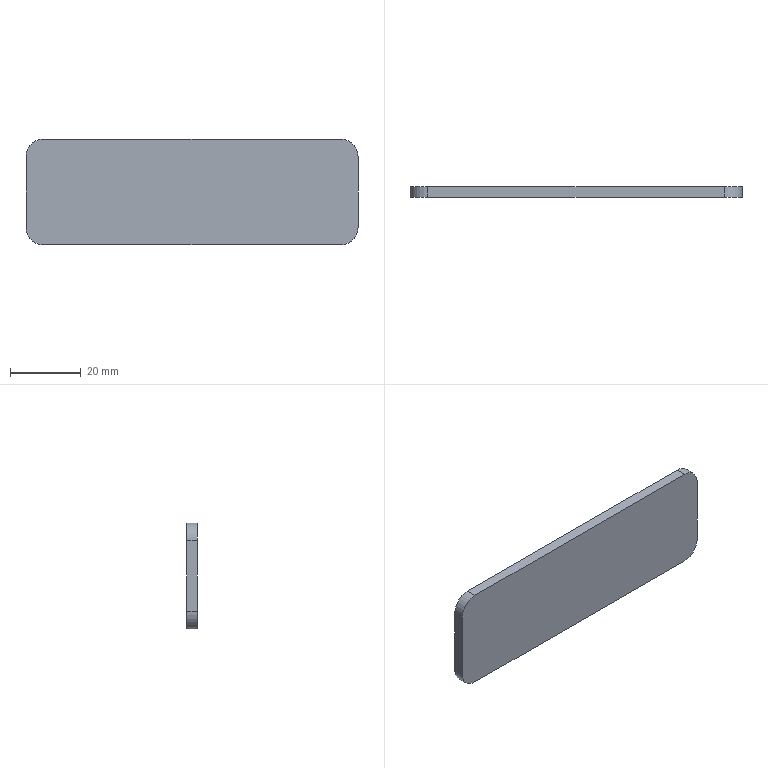Part | SolidWorks | features Extrusion 1, Fillet 1 | 1 solid | 10 faces | box 94 x 3 x 30 mm | volume 8396 mm3 | plane 6 | cylinder 4 | commonest cylinder face diameters 10 x4
STEP:
#1=CARTESIAN_POINT('',(47.,3.,10.));
#2=VERTEX_POINT('',#1);
#3=CARTESIAN_POINT('',(47.,3.,-10.));
#4=VERTEX_POINT('',#3);
#5=CARTESIAN_POINT('',(47.,3.,15.));
#6=DIRECTION('',(0.,0.,-1.));
#7=VECTOR('',#6,1000.);
#8=LINE('',#5,#7);
#9=EDGE_CURVE('',#2,#4,#8,.T.);
#10=ORIENTED_EDGE('',*,*,#9,.F.);
#11=CARTESIAN_POINT('',(47.,0.,10.));
#12=VERTEX_POINT('',#11);
#13=CARTESIAN_POINT('',(47.,3.,10.));
#14=DIRECTION('',(0.,-1.,0.));
#15=VECTOR('',#14,1000.);
#16=LINE('',#13,#15);
#17=EDGE_CURVE('',#2,#12,#16,.T.);
#18=ORIENTED_EDGE('',*,*,#17,.T.);
#19=CARTESIAN_POINT('',(47.,0.,-10.));
#20=VERTEX_POINT('',#19);
#21=CARTESIAN_POINT('',(47.,0.,15.));
#22=DIRECTION('',(0.,0.,-1.));
#23=VECTOR('',#22,1000.);
#24=LINE('',#21,#23);
#25=EDGE_CURVE('',#12,#20,#24,.T.);
#26=ORIENTED_EDGE('',*,*,#25,.T.);
#27=CARTESIAN_POINT('',(47.,3.,-10.));
#28=DIRECTION('',(0.,1.,0.));
#29=VECTOR('',#28,1000.);
#30=LINE('',#27,#29);
#31=EDGE_CURVE('',#20,#4,#30,.T.);
#32=ORIENTED_EDGE('',*,*,#31,.T.);
#33=EDGE_LOOP('',(#10,#18,#26,#32));
#34=FACE_OUTER_BOUND('',#33,.T.);
#35=CARTESIAN_POINT('',(47.,3.,15.));
#36=DIRECTION('',(-1.,0.,0.));
#37=DIRECTION('',(0.,0.,1.));
#38=AXIS2_PLACEMENT_3D('',#35,#36,#37);
#39=PLANE('',#38);
#40=ADVANCED_FACE('',(#34),#39,.F.);
#41=CARTESIAN_POINT('',(42.,3.,-15.));
#42=VERTEX_POINT('',#41);
#43=CARTESIAN_POINT('',(-42.,3.,-15.));
#44=VERTEX_POINT('',#43);
#45=CARTESIAN_POINT('',(-47.,3.,-15.));
#46=DIRECTION('',(-1.,0.,0.));
#47=VECTOR('',#46,1000.);
#48=LINE('',#45,#47);
#49=EDGE_CURVE('',#42,#44,#48,.T.);
#50=ORIENTED_EDGE('',*,*,#49,.F.);
#51=CARTESIAN_POINT('',(42.,0.,-15.));
#52=VERTEX_POINT('',#51);
#53=CARTESIAN_POINT('',(42.,3.,-15.));
#54=DIRECTION('',(0.,-1.,0.));
#55=VECTOR('',#54,1000.);
#56=LINE('',#53,#55);
#57=EDGE_CURVE('',#42,#52,#56,.T.);
#58=ORIENTED_EDGE('',*,*,#57,.T.);
#59=CARTESIAN_POINT('',(-42.,0.,-15.));
#60=VERTEX_POINT('',#59);
#61=CARTESIAN_POINT('',(-47.,0.,-15.));
#62=DIRECTION('',(-1.,0.,0.));
#63=VECTOR('',#62,1000.);
#64=LINE('',#61,#63);
#65=EDGE_CURVE('',#52,#60,#64,.T.);
#66=ORIENTED_EDGE('',*,*,#65,.T.);
#67=CARTESIAN_POINT('',(-42.,3.,-15.));
#68=DIRECTION('',(0.,1.,0.));
#69=VECTOR('',#68,1000.);
#70=LINE('',#67,#69);
#71=EDGE_CURVE('',#60,#44,#70,.T.);
#72=ORIENTED_EDGE('',*,*,#71,.T.);
#73=EDGE_LOOP('',(#50,#58,#66,#72));
#74=FACE_OUTER_BOUND('',#73,.T.);
#75=CARTESIAN_POINT('',(-47.,3.,-15.));
#76=DIRECTION('',(0.,0.,1.));
#77=DIRECTION('',(1.,0.,0.));
#78=AXIS2_PLACEMENT_3D('',#75,#76,#77);
#79=PLANE('',#78);
#80=ADVANCED_FACE('',(#74),#79,.F.);
#81=CARTESIAN_POINT('',(-47.,3.,-10.));
#82=VERTEX_POINT('',#81);
#83=CARTESIAN_POINT('',(-47.,3.,10.));
#84=VERTEX_POINT('',#83);
#85=CARTESIAN_POINT('',(-47.,3.,15.));
#86=DIRECTION('',(0.,0.,1.));
#87=VECTOR('',#86,1000.);
#88=LINE('',#85,#87);
#89=EDGE_CURVE('',#82,#84,#88,.T.);
#90=ORIENTED_EDGE('',*,*,#89,.F.);
#91=CARTESIAN_POINT('',(-47.,0.,-10.));
#92=VERTEX_POINT('',#91);
#93=CARTESIAN_POINT('',(-47.,3.,-10.));
#94=DIRECTION('',(0.,-1.,0.));
#95=VECTOR('',#94,1000.);
#96=LINE('',#93,#95);
#97=EDGE_CURVE('',#82,#92,#96,.T.);
#98=ORIENTED_EDGE('',*,*,#97,.T.);
#99=CARTESIAN_POINT('',(-47.,0.,10.));
#100=VERTEX_POINT('',#99);
#101=CARTESIAN_POINT('',(-47.,0.,15.));
#102=DIRECTION('',(0.,0.,1.));
#103=VECTOR('',#102,1000.);
#104=LINE('',#101,#103);
#105=EDGE_CURVE('',#92,#100,#104,.T.);
#106=ORIENTED_EDGE('',*,*,#105,.T.);
#107=CARTESIAN_POINT('',(-47.,3.,10.));
#108=DIRECTION('',(0.,1.,0.));
#109=VECTOR('',#108,1000.);
#110=LINE('',#107,#109);
#111=EDGE_CURVE('',#100,#84,#110,.T.);
#112=ORIENTED_EDGE('',*,*,#111,.T.);
#113=EDGE_LOOP('',(#90,#98,#106,#112));
#114=FACE_OUTER_BOUND('',#113,.T.);
#115=CARTESIAN_POINT('',(-47.,3.,15.));
#116=DIRECTION('',(1.,0.,0.));
#117=DIRECTION('',(0.,0.,-1.));
#118=AXIS2_PLACEMENT_3D('',#115,#116,#117);
#119=PLANE('',#118);
#120=ADVANCED_FACE('',(#114),#119,.F.);
#121=CARTESIAN_POINT('',(-42.,0.,15.));
#122=VERTEX_POINT('',#121);
#123=CARTESIAN_POINT('',(42.,0.,15.));
#124=VERTEX_POINT('',#123);
#125=CARTESIAN_POINT('',(-47.,0.,15.));
#126=DIRECTION('',(1.,0.,0.));
#127=VECTOR('',#126,1000.);
#128=LINE('',#125,#127);
#129=EDGE_CURVE('',#122,#124,#128,.T.);
#130=ORIENTED_EDGE('',*,*,#129,.T.);
#131=CARTESIAN_POINT('',(42.,3.,15.));
#132=VERTEX_POINT('',#131);
#133=CARTESIAN_POINT('',(42.,3.,15.));
#134=DIRECTION('',(0.,1.,0.));
#135=VECTOR('',#134,1000.);
#136=LINE('',#133,#135);
#137=EDGE_CURVE('',#124,#132,#136,.T.);
#138=ORIENTED_EDGE('',*,*,#137,.T.);
#139=CARTESIAN_POINT('',(-42.,3.,15.));
#140=VERTEX_POINT('',#139);
#141=CARTESIAN_POINT('',(-47.,3.,15.));
#142=DIRECTION('',(1.,0.,0.));
#143=VECTOR('',#142,1000.);
#144=LINE('',#141,#143);
#145=EDGE_CURVE('',#140,#132,#144,.T.);
#146=ORIENTED_EDGE('',*,*,#145,.F.);
#147=CARTESIAN_POINT('',(-42.,3.,15.));
#148=DIRECTION('',(0.,-1.,0.));
#149=VECTOR('',#148,1000.);
#150=LINE('',#147,#149);
#151=EDGE_CURVE('',#140,#122,#150,.T.);
#152=ORIENTED_EDGE('',*,*,#151,.T.);
#153=EDGE_LOOP('',(#130,#138,#146,#152));
#154=FACE_OUTER_BOUND('',#153,.T.);
#155=CARTESIAN_POINT('',(-47.,3.,15.));
#156=DIRECTION('',(0.,0.,-1.));
#157=DIRECTION('',(-1.,0.,0.));
#158=AXIS2_PLACEMENT_3D('',#155,#156,#157);
#159=PLANE('',#158);
#160=ADVANCED_FACE('',(#154),#159,.F.);
#161=ORIENTED_EDGE('',*,*,#145,.T.);
#162=CARTESIAN_POINT('',(42.,3.,10.));
#163=DIRECTION('',(0.,1.,0.));
#164=DIRECTION('',(0.,0.,-1.));
#165=AXIS2_PLACEMENT_3D('',#162,#163,#164);
#166=CIRCLE('',#165,5.);
#167=EDGE_CURVE('',#132,#2,#166,.T.);
#168=ORIENTED_EDGE('',*,*,#167,.T.);
#169=ORIENTED_EDGE('',*,*,#9,.T.);
#170=CARTESIAN_POINT('',(42.,3.,-10.));
#171=DIRECTION('',(0.,1.,0.));
#172=DIRECTION('',(0.,0.,-1.));
#173=AXIS2_PLACEMENT_3D('',#170,#171,#172);
#174=CIRCLE('',#173,5.);
#175=EDGE_CURVE('',#4,#42,#174,.T.);
#176=ORIENTED_EDGE('',*,*,#175,.T.);
#177=ORIENTED_EDGE('',*,*,#49,.T.);
#178=CARTESIAN_POINT('',(-42.,3.,-10.));
#179=DIRECTION('',(0.,1.,0.));
#180=DIRECTION('',(0.,0.,-1.));
#181=AXIS2_PLACEMENT_3D('',#178,#179,#180);
#182=CIRCLE('',#181,5.);
#183=EDGE_CURVE('',#44,#82,#182,.T.);
#184=ORIENTED_EDGE('',*,*,#183,.T.);
#185=ORIENTED_EDGE('',*,*,#89,.T.);
#186=CARTESIAN_POINT('',(-42.,3.,10.));
#187=DIRECTION('',(0.,1.,0.));
#188=DIRECTION('',(0.,0.,-1.));
#189=AXIS2_PLACEMENT_3D('',#186,#187,#188);
#190=CIRCLE('',#189,5.);
#191=EDGE_CURVE('',#84,#140,#190,.T.);
#192=ORIENTED_EDGE('',*,*,#191,.T.);
#193=EDGE_LOOP('',(#161,#168,#169,#176,#177,#184,#185,#192));
#194=FACE_OUTER_BOUND('',#193,.T.);
#195=CARTESIAN_POINT('',(0.,3.,0.));
#196=DIRECTION('',(0.,-1.,0.));
#197=DIRECTION('',(0.,0.,-1.));
#198=AXIS2_PLACEMENT_3D('',#195,#196,#197);
#199=PLANE('',#198);
#200=ADVANCED_FACE('',(#194),#199,.F.);
#201=ORIENTED_EDGE('',*,*,#25,.F.);
#202=CARTESIAN_POINT('',(42.,0.,10.));
#203=DIRECTION('',(0.,-1.,0.));
#204=DIRECTION('',(0.,0.,-1.));
#205=AXIS2_PLACEMENT_3D('',#202,#203,#204);
#206=CIRCLE('',#205,5.);
#207=EDGE_CURVE('',#12,#124,#206,.T.);
#208=ORIENTED_EDGE('',*,*,#207,.T.);
#209=ORIENTED_EDGE('',*,*,#129,.F.);
#210=CARTESIAN_POINT('',(-42.,0.,10.));
#211=DIRECTION('',(0.,-1.,0.));
#212=DIRECTION('',(0.,0.,-1.));
#213=AXIS2_PLACEMENT_3D('',#210,#211,#212);
#214=CIRCLE('',#213,5.);
#215=EDGE_CURVE('',#122,#100,#214,.T.);
#216=ORIENTED_EDGE('',*,*,#215,.T.);
#217=ORIENTED_EDGE('',*,*,#105,.F.);
#218=CARTESIAN_POINT('',(-42.,0.,-10.));
#219=DIRECTION('',(0.,-1.,0.));
#220=DIRECTION('',(0.,0.,-1.));
#221=AXIS2_PLACEMENT_3D('',#218,#219,#220);
#222=CIRCLE('',#221,5.);
#223=EDGE_CURVE('',#92,#60,#222,.T.);
#224=ORIENTED_EDGE('',*,*,#223,.T.);
#225=ORIENTED_EDGE('',*,*,#65,.F.);
#226=CARTESIAN_POINT('',(42.,0.,-10.));
#227=DIRECTION('',(0.,-1.,0.));
#228=DIRECTION('',(0.,0.,-1.));
#229=AXIS2_PLACEMENT_3D('',#226,#227,#228);
#230=CIRCLE('',#229,5.);
#231=EDGE_CURVE('',#52,#20,#230,.T.);
#232=ORIENTED_EDGE('',*,*,#231,.T.);
#233=EDGE_LOOP('',(#201,#208,#209,#216,#217,#224,#225,#232));
#234=FACE_OUTER_BOUND('',#233,.T.);
#235=CARTESIAN_POINT('',(0.,0.,0.));
#236=DIRECTION('',(0.,-1.,0.));
#237=DIRECTION('',(0.,0.,-1.));
#238=AXIS2_PLACEMENT_3D('',#235,#236,#237);
#239=PLANE('',#238);
#240=ADVANCED_FACE('',(#234),#239,.T.);
#241=ORIENTED_EDGE('',*,*,#167,.F.);
#242=ORIENTED_EDGE('',*,*,#137,.F.);
#243=ORIENTED_EDGE('',*,*,#207,.F.);
#244=ORIENTED_EDGE('',*,*,#17,.F.);
#245=EDGE_LOOP('',(#241,#242,#243,#244));
#246=FACE_OUTER_BOUND('',#245,.T.);
#247=CARTESIAN_POINT('',(42.,3.,10.));
#248=DIRECTION('',(0.,-1.,0.));
#249=DIRECTION('',(0.,0.,-1.));
#250=AXIS2_PLACEMENT_3D('',#247,#248,#249);
#251=CYLINDRICAL_SURFACE('',#250,5.);
#252=ADVANCED_FACE('',(#246),#251,.T.);
#253=ORIENTED_EDGE('',*,*,#175,.F.);
#254=ORIENTED_EDGE('',*,*,#31,.F.);
#255=ORIENTED_EDGE('',*,*,#231,.F.);
#256=ORIENTED_EDGE('',*,*,#57,.F.);
#257=EDGE_LOOP('',(#253,#254,#255,#256));
#258=FACE_OUTER_BOUND('',#257,.T.);
#259=CARTESIAN_POINT('',(42.,3.,-10.));
#260=DIRECTION('',(0.,-1.,0.));
#261=DIRECTION('',(0.,0.,-1.));
#262=AXIS2_PLACEMENT_3D('',#259,#260,#261);
#263=CYLINDRICAL_SURFACE('',#262,5.);
#264=ADVANCED_FACE('',(#258),#263,.T.);
#265=ORIENTED_EDGE('',*,*,#183,.F.);
#266=ORIENTED_EDGE('',*,*,#71,.F.);
#267=ORIENTED_EDGE('',*,*,#223,.F.);
#268=ORIENTED_EDGE('',*,*,#97,.F.);
#269=EDGE_LOOP('',(#265,#266,#267,#268));
#270=FACE_OUTER_BOUND('',#269,.T.);
#271=CARTESIAN_POINT('',(-42.,3.,-10.));
#272=DIRECTION('',(0.,-1.,0.));
#273=DIRECTION('',(0.,0.,-1.));
#274=AXIS2_PLACEMENT_3D('',#271,#272,#273);
#275=CYLINDRICAL_SURFACE('',#274,5.);
#276=ADVANCED_FACE('',(#270),#275,.T.);
#277=ORIENTED_EDGE('',*,*,#191,.F.);
#278=ORIENTED_EDGE('',*,*,#111,.F.);
#279=ORIENTED_EDGE('',*,*,#215,.F.);
#280=ORIENTED_EDGE('',*,*,#151,.F.);
#281=EDGE_LOOP('',(#277,#278,#279,#280));
#282=FACE_OUTER_BOUND('',#281,.T.);
#283=CARTESIAN_POINT('',(-42.,3.,10.));
#284=DIRECTION('',(0.,-1.,0.));
#285=DIRECTION('',(0.,0.,-1.));
#286=AXIS2_PLACEMENT_3D('',#283,#284,#285);
#287=CYLINDRICAL_SURFACE('',#286,5.);
#288=ADVANCED_FACE('',(#282),#287,.T.);
#289=CLOSED_SHELL('',(#40,#80,#120,#160,#200,#240,#252,#264,#276,#288));
#290=MANIFOLD_SOLID_BREP('',#289);
#291=CARTESIAN_POINT('',(0.,0.,0.));
#292=DIRECTION('',(0.,0.,1.));
#293=DIRECTION('',(1.,0.,0.));
#294=AXIS2_PLACEMENT_3D('',#291,#292,#293);
#295=(LENGTH_UNIT()NAMED_UNIT(*)SI_UNIT(.MILLI.,.METRE.));
#296=UNCERTAINTY_MEASURE_WITH_UNIT(LENGTH_MEASURE(0.00001),#295,'','');
#297=(NAMED_UNIT(*)PLANE_ANGLE_UNIT()SI_UNIT($,.RADIAN.));
#298=(NAMED_UNIT(*)SI_UNIT($,.STERADIAN.)SOLID_ANGLE_UNIT());
#299=(GEOMETRIC_REPRESENTATION_CONTEXT(3)GLOBAL_UNCERTAINTY_ASSIGNED_CONTEXT((#296))GLOBAL_UNIT_ASSIGNED_CONTEXT((#295,#297,#298))REPRESENTATION_CONTEXT('',''));
#300=ADVANCED_BREP_SHAPE_REPRESENTATION('',(#290,#294),#299);